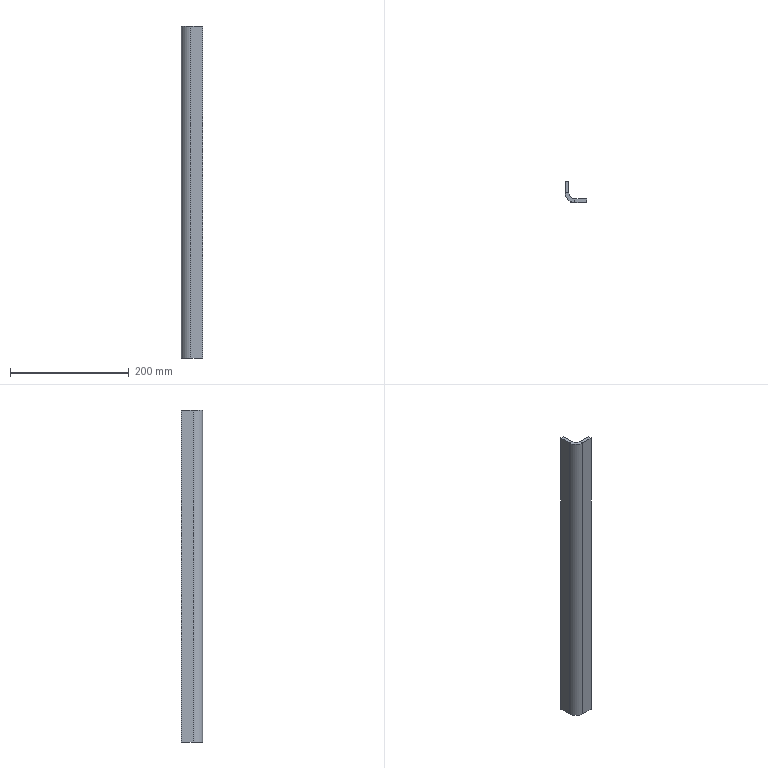Part | SolidWorks | features FlatPattern 1, SMBaseFlange 1, SheetMetal 1 | 1 solid | 14 faces | box 36 x 36 x 560 mm | volume 203012 mm3 | plane 12 | cylinder 2 | commonest cylinder face diameters 20 x1 32 x1
STEP:
#1=CARTESIAN_POINT('',(0.,16.,560.));
#2=VERTEX_POINT('',#1);
#3=CARTESIAN_POINT('',(6.,16.,560.));
#4=VERTEX_POINT('',#3);
#5=CARTESIAN_POINT('',(0.,16.,560.));
#6=DIRECTION('',(1.,0.,0.));
#7=VECTOR('',#6,1000.);
#8=LINE('',#5,#7);
#9=EDGE_CURVE('',#2,#4,#8,.T.);
#10=ORIENTED_EDGE('',*,*,#9,.F.);
#11=CARTESIAN_POINT('',(16.,0.,560.));
#12=VERTEX_POINT('',#11);
#13=CARTESIAN_POINT('',(16.,16.,560.));
#14=DIRECTION('',(0.,0.,1.));
#15=DIRECTION('',(-1.,0.,0.));
#16=AXIS2_PLACEMENT_3D('',#13,#14,#15);
#17=CIRCLE('',#16,16.);
#18=EDGE_CURVE('',#2,#12,#17,.T.);
#19=ORIENTED_EDGE('',*,*,#18,.T.);
#20=CARTESIAN_POINT('',(16.,6.,560.));
#21=VERTEX_POINT('',#20);
#22=CARTESIAN_POINT('',(16.,6.,560.));
#23=DIRECTION('',(0.,-1.,0.));
#24=VECTOR('',#23,1000.);
#25=LINE('',#22,#24);
#26=EDGE_CURVE('',#21,#12,#25,.T.);
#27=ORIENTED_EDGE('',*,*,#26,.F.);
#28=CARTESIAN_POINT('',(16.,16.,560.));
#29=DIRECTION('',(0.,0.,1.));
#30=DIRECTION('',(1.,0.,0.));
#31=AXIS2_PLACEMENT_3D('',#28,#29,#30);
#32=CIRCLE('',#31,10.);
#33=EDGE_CURVE('',#4,#21,#32,.T.);
#34=ORIENTED_EDGE('',*,*,#33,.F.);
#35=EDGE_LOOP('',(#10,#19,#27,#34));
#36=FACE_OUTER_BOUND('',#35,.T.);
#37=CARTESIAN_POINT('',(0.,16.,560.));
#38=DIRECTION('',(0.,0.,1.));
#39=DIRECTION('',(1.,0.,0.));
#40=AXIS2_PLACEMENT_3D('',#37,#38,#39);
#41=PLANE('',#40);
#42=ADVANCED_FACE('',(#36),#41,.T.);
#43=CARTESIAN_POINT('',(0.,36.,560.));
#44=VERTEX_POINT('',#43);
#45=CARTESIAN_POINT('',(0.,0.,560.));
#46=DIRECTION('',(0.,-1.,0.));
#47=VECTOR('',#46,1000.);
#48=LINE('',#45,#47);
#49=EDGE_CURVE('',#44,#2,#48,.T.);
#50=ORIENTED_EDGE('',*,*,#49,.T.);
#51=ORIENTED_EDGE('',*,*,#9,.T.);
#52=CARTESIAN_POINT('',(6.,36.,560.));
#53=VERTEX_POINT('',#52);
#54=CARTESIAN_POINT('',(6.,0.,560.));
#55=DIRECTION('',(0.,-1.,0.));
#56=VECTOR('',#55,1000.);
#57=LINE('',#54,#56);
#58=EDGE_CURVE('',#53,#4,#57,.T.);
#59=ORIENTED_EDGE('',*,*,#58,.F.);
#60=CARTESIAN_POINT('',(0.,36.,560.));
#61=DIRECTION('',(1.,0.,0.));
#62=VECTOR('',#61,1000.);
#63=LINE('',#60,#62);
#64=EDGE_CURVE('',#44,#53,#63,.T.);
#65=ORIENTED_EDGE('',*,*,#64,.F.);
#66=EDGE_LOOP('',(#50,#51,#59,#65));
#67=FACE_OUTER_BOUND('',#66,.T.);
#68=CARTESIAN_POINT('',(16.,6.,560.));
#69=DIRECTION('',(0.,0.,1.));
#70=DIRECTION('',(1.,0.,0.));
#71=AXIS2_PLACEMENT_3D('',#68,#69,#70);
#72=PLANE('',#71);
#73=ADVANCED_FACE('',(#67),#72,.T.);
#74=CARTESIAN_POINT('',(16.,0.,0.));
#75=VERTEX_POINT('',#74);
#76=CARTESIAN_POINT('',(16.,6.,0.));
#77=VERTEX_POINT('',#76);
#78=CARTESIAN_POINT('',(16.,0.,0.));
#79=DIRECTION('',(0.,1.,0.));
#80=VECTOR('',#79,1000.);
#81=LINE('',#78,#80);
#82=EDGE_CURVE('',#75,#77,#81,.T.);
#83=ORIENTED_EDGE('',*,*,#82,.F.);
#84=CARTESIAN_POINT('',(0.,16.,0.));
#85=VERTEX_POINT('',#84);
#86=CARTESIAN_POINT('',(16.,16.,0.));
#87=DIRECTION('',(0.,0.,1.));
#88=DIRECTION('',(-1.,0.,0.));
#89=AXIS2_PLACEMENT_3D('',#86,#87,#88);
#90=CIRCLE('',#89,16.);
#91=EDGE_CURVE('',#85,#75,#90,.T.);
#92=ORIENTED_EDGE('',*,*,#91,.F.);
#93=CARTESIAN_POINT('',(6.,16.,0.));
#94=VERTEX_POINT('',#93);
#95=CARTESIAN_POINT('',(6.,16.,0.));
#96=DIRECTION('',(-1.,0.,0.));
#97=VECTOR('',#96,1000.);
#98=LINE('',#95,#97);
#99=EDGE_CURVE('',#94,#85,#98,.T.);
#100=ORIENTED_EDGE('',*,*,#99,.F.);
#101=CARTESIAN_POINT('',(16.,16.,0.));
#102=DIRECTION('',(0.,0.,1.));
#103=DIRECTION('',(1.,0.,0.));
#104=AXIS2_PLACEMENT_3D('',#101,#102,#103);
#105=CIRCLE('',#104,10.);
#106=EDGE_CURVE('',#94,#77,#105,.T.);
#107=ORIENTED_EDGE('',*,*,#106,.T.);
#108=EDGE_LOOP('',(#83,#92,#100,#107));
#109=FACE_OUTER_BOUND('',#108,.T.);
#110=CARTESIAN_POINT('',(16.,0.,0.));
#111=DIRECTION('',(0.,0.,-1.));
#112=DIRECTION('',(-1.,0.,0.));
#113=AXIS2_PLACEMENT_3D('',#110,#111,#112);
#114=PLANE('',#113);
#115=ADVANCED_FACE('',(#109),#114,.T.);
#116=CARTESIAN_POINT('',(36.,0.,0.));
#117=VERTEX_POINT('',#116);
#118=CARTESIAN_POINT('',(0.,0.,0.));
#119=DIRECTION('',(1.,0.,0.));
#120=VECTOR('',#119,1000.);
#121=LINE('',#118,#120);
#122=EDGE_CURVE('',#75,#117,#121,.T.);
#123=ORIENTED_EDGE('',*,*,#122,.F.);
#124=ORIENTED_EDGE('',*,*,#82,.T.);
#125=CARTESIAN_POINT('',(36.,6.,0.));
#126=VERTEX_POINT('',#125);
#127=CARTESIAN_POINT('',(0.,6.,0.));
#128=DIRECTION('',(1.,0.,0.));
#129=VECTOR('',#128,1000.);
#130=LINE('',#127,#129);
#131=EDGE_CURVE('',#77,#126,#130,.T.);
#132=ORIENTED_EDGE('',*,*,#131,.T.);
#133=CARTESIAN_POINT('',(36.,6.,0.));
#134=DIRECTION('',(0.,-1.,0.));
#135=VECTOR('',#134,1000.);
#136=LINE('',#133,#135);
#137=EDGE_CURVE('',#126,#117,#136,.T.);
#138=ORIENTED_EDGE('',*,*,#137,.T.);
#139=EDGE_LOOP('',(#123,#124,#132,#138));
#140=FACE_OUTER_BOUND('',#139,.T.);
#141=CARTESIAN_POINT('',(6.,16.,0.));
#142=DIRECTION('',(0.,0.,-1.));
#143=DIRECTION('',(-1.,0.,0.));
#144=AXIS2_PLACEMENT_3D('',#141,#142,#143);
#145=PLANE('',#144);
#146=ADVANCED_FACE('',(#140),#145,.T.);
#147=ORIENTED_EDGE('',*,*,#122,.T.);
#148=CARTESIAN_POINT('',(36.,0.,560.));
#149=VERTEX_POINT('',#148);
#150=CARTESIAN_POINT('',(36.,0.,560.));
#151=DIRECTION('',(0.,0.,-1.));
#152=VECTOR('',#151,1000.);
#153=LINE('',#150,#152);
#154=EDGE_CURVE('',#149,#117,#153,.T.);
#155=ORIENTED_EDGE('',*,*,#154,.F.);
#156=CARTESIAN_POINT('',(0.,0.,560.));
#157=DIRECTION('',(1.,0.,0.));
#158=VECTOR('',#157,1000.);
#159=LINE('',#156,#158);
#160=EDGE_CURVE('',#12,#149,#159,.T.);
#161=ORIENTED_EDGE('',*,*,#160,.F.);
#162=CARTESIAN_POINT('',(16.,0.,560.));
#163=DIRECTION('',(0.,0.,-1.));
#164=VECTOR('',#163,1000.);
#165=LINE('',#162,#164);
#166=EDGE_CURVE('',#12,#75,#165,.T.);
#167=ORIENTED_EDGE('',*,*,#166,.T.);
#168=EDGE_LOOP('',(#147,#155,#161,#167));
#169=FACE_OUTER_BOUND('',#168,.T.);
#170=CARTESIAN_POINT('',(0.,0.,560.));
#171=DIRECTION('',(0.,1.,0.));
#172=DIRECTION('',(0.,0.,1.));
#173=AXIS2_PLACEMENT_3D('',#170,#171,#172);
#174=PLANE('',#173);
#175=ADVANCED_FACE('',(#169),#174,.F.);
#176=ORIENTED_EDGE('',*,*,#137,.F.);
#177=CARTESIAN_POINT('',(36.,6.,560.));
#178=VERTEX_POINT('',#177);
#179=CARTESIAN_POINT('',(36.,6.,560.));
#180=DIRECTION('',(0.,0.,-1.));
#181=VECTOR('',#180,1000.);
#182=LINE('',#179,#181);
#183=EDGE_CURVE('',#178,#126,#182,.T.);
#184=ORIENTED_EDGE('',*,*,#183,.F.);
#185=CARTESIAN_POINT('',(36.,6.,560.));
#186=DIRECTION('',(0.,-1.,0.));
#187=VECTOR('',#186,1000.);
#188=LINE('',#185,#187);
#189=EDGE_CURVE('',#178,#149,#188,.T.);
#190=ORIENTED_EDGE('',*,*,#189,.T.);
#191=ORIENTED_EDGE('',*,*,#154,.T.);
#192=EDGE_LOOP('',(#176,#184,#190,#191));
#193=FACE_OUTER_BOUND('',#192,.T.);
#194=CARTESIAN_POINT('',(36.,6.,560.));
#195=DIRECTION('',(1.,0.,0.));
#196=DIRECTION('',(0.,0.,-1.));
#197=AXIS2_PLACEMENT_3D('',#194,#195,#196);
#198=PLANE('',#197);
#199=ADVANCED_FACE('',(#193),#198,.T.);
#200=ORIENTED_EDGE('',*,*,#131,.F.);
#201=CARTESIAN_POINT('',(16.,6.,560.));
#202=DIRECTION('',(0.,0.,-1.));
#203=VECTOR('',#202,1000.);
#204=LINE('',#201,#203);
#205=EDGE_CURVE('',#21,#77,#204,.T.);
#206=ORIENTED_EDGE('',*,*,#205,.F.);
#207=CARTESIAN_POINT('',(0.,6.,560.));
#208=DIRECTION('',(1.,0.,0.));
#209=VECTOR('',#208,1000.);
#210=LINE('',#207,#209);
#211=EDGE_CURVE('',#21,#178,#210,.T.);
#212=ORIENTED_EDGE('',*,*,#211,.T.);
#213=ORIENTED_EDGE('',*,*,#183,.T.);
#214=EDGE_LOOP('',(#200,#206,#212,#213));
#215=FACE_OUTER_BOUND('',#214,.T.);
#216=CARTESIAN_POINT('',(0.,6.,560.));
#217=DIRECTION('',(0.,1.,0.));
#218=DIRECTION('',(0.,0.,1.));
#219=AXIS2_PLACEMENT_3D('',#216,#217,#218);
#220=PLANE('',#219);
#221=ADVANCED_FACE('',(#215),#220,.T.);
#222=ORIENTED_EDGE('',*,*,#106,.F.);
#223=CARTESIAN_POINT('',(6.,16.,560.));
#224=DIRECTION('',(0.,0.,-1.));
#225=VECTOR('',#224,1000.);
#226=LINE('',#223,#225);
#227=EDGE_CURVE('',#4,#94,#226,.T.);
#228=ORIENTED_EDGE('',*,*,#227,.F.);
#229=ORIENTED_EDGE('',*,*,#33,.T.);
#230=ORIENTED_EDGE('',*,*,#205,.T.);
#231=EDGE_LOOP('',(#222,#228,#229,#230));
#232=FACE_OUTER_BOUND('',#231,.T.);
#233=CARTESIAN_POINT('',(16.,16.,560.));
#234=DIRECTION('',(0.,0.,-1.));
#235=DIRECTION('',(-1.,0.,0.));
#236=AXIS2_PLACEMENT_3D('',#233,#234,#235);
#237=CYLINDRICAL_SURFACE('',#236,10.);
#238=ADVANCED_FACE('',(#232),#237,.F.);
#239=CARTESIAN_POINT('',(6.,36.,0.));
#240=VERTEX_POINT('',#239);
#241=CARTESIAN_POINT('',(6.,0.,0.));
#242=DIRECTION('',(0.,-1.,0.));
#243=VECTOR('',#242,1000.);
#244=LINE('',#241,#243);
#245=EDGE_CURVE('',#240,#94,#244,.T.);
#246=ORIENTED_EDGE('',*,*,#245,.F.);
#247=CARTESIAN_POINT('',(6.,36.,560.));
#248=DIRECTION('',(0.,0.,-1.));
#249=VECTOR('',#248,1000.);
#250=LINE('',#247,#249);
#251=EDGE_CURVE('',#53,#240,#250,.T.);
#252=ORIENTED_EDGE('',*,*,#251,.F.);
#253=ORIENTED_EDGE('',*,*,#58,.T.);
#254=ORIENTED_EDGE('',*,*,#227,.T.);
#255=EDGE_LOOP('',(#246,#252,#253,#254));
#256=FACE_OUTER_BOUND('',#255,.T.);
#257=CARTESIAN_POINT('',(6.,0.,560.));
#258=DIRECTION('',(1.,0.,0.));
#259=DIRECTION('',(0.,0.,-1.));
#260=AXIS2_PLACEMENT_3D('',#257,#258,#259);
#261=PLANE('',#260);
#262=ADVANCED_FACE('',(#256),#261,.T.);
#263=CARTESIAN_POINT('',(0.,36.,0.));
#264=VERTEX_POINT('',#263);
#265=CARTESIAN_POINT('',(0.,36.,0.));
#266=DIRECTION('',(1.,0.,0.));
#267=VECTOR('',#266,1000.);
#268=LINE('',#265,#267);
#269=EDGE_CURVE('',#264,#240,#268,.T.);
#270=ORIENTED_EDGE('',*,*,#269,.F.);
#271=CARTESIAN_POINT('',(0.,36.,560.));
#272=DIRECTION('',(0.,0.,-1.));
#273=VECTOR('',#272,1000.);
#274=LINE('',#271,#273);
#275=EDGE_CURVE('',#44,#264,#274,.T.);
#276=ORIENTED_EDGE('',*,*,#275,.F.);
#277=ORIENTED_EDGE('',*,*,#64,.T.);
#278=ORIENTED_EDGE('',*,*,#251,.T.);
#279=EDGE_LOOP('',(#270,#276,#277,#278));
#280=FACE_OUTER_BOUND('',#279,.T.);
#281=CARTESIAN_POINT('',(0.,36.,560.));
#282=DIRECTION('',(0.,1.,0.));
#283=DIRECTION('',(0.,0.,1.));
#284=AXIS2_PLACEMENT_3D('',#281,#282,#283);
#285=PLANE('',#284);
#286=ADVANCED_FACE('',(#280),#285,.T.);
#287=CARTESIAN_POINT('',(0.,0.,0.));
#288=DIRECTION('',(0.,-1.,0.));
#289=VECTOR('',#288,1000.);
#290=LINE('',#287,#289);
#291=EDGE_CURVE('',#264,#85,#290,.T.);
#292=ORIENTED_EDGE('',*,*,#291,.T.);
#293=CARTESIAN_POINT('',(0.,16.,560.));
#294=DIRECTION('',(0.,0.,-1.));
#295=VECTOR('',#294,1000.);
#296=LINE('',#293,#295);
#297=EDGE_CURVE('',#2,#85,#296,.T.);
#298=ORIENTED_EDGE('',*,*,#297,.F.);
#299=ORIENTED_EDGE('',*,*,#49,.F.);
#300=ORIENTED_EDGE('',*,*,#275,.T.);
#301=EDGE_LOOP('',(#292,#298,#299,#300));
#302=FACE_OUTER_BOUND('',#301,.T.);
#303=CARTESIAN_POINT('',(0.,0.,560.));
#304=DIRECTION('',(1.,0.,0.));
#305=DIRECTION('',(0.,0.,-1.));
#306=AXIS2_PLACEMENT_3D('',#303,#304,#305);
#307=PLANE('',#306);
#308=ADVANCED_FACE('',(#302),#307,.F.);
#309=ORIENTED_EDGE('',*,*,#91,.T.);
#310=ORIENTED_EDGE('',*,*,#166,.F.);
#311=ORIENTED_EDGE('',*,*,#18,.F.);
#312=ORIENTED_EDGE('',*,*,#297,.T.);
#313=EDGE_LOOP('',(#309,#310,#311,#312));
#314=FACE_OUTER_BOUND('',#313,.T.);
#315=CARTESIAN_POINT('',(16.,16.,560.));
#316=DIRECTION('',(0.,0.,-1.));
#317=DIRECTION('',(-1.,0.,0.));
#318=AXIS2_PLACEMENT_3D('',#315,#316,#317);
#319=CYLINDRICAL_SURFACE('',#318,16.);
#320=ADVANCED_FACE('',(#314),#319,.T.);
#321=ORIENTED_EDGE('',*,*,#160,.T.);
#322=ORIENTED_EDGE('',*,*,#189,.F.);
#323=ORIENTED_EDGE('',*,*,#211,.F.);
#324=ORIENTED_EDGE('',*,*,#26,.T.);
#325=EDGE_LOOP('',(#321,#322,#323,#324));
#326=FACE_OUTER_BOUND('',#325,.T.);
#327=CARTESIAN_POINT('',(16.,16.,560.));
#328=DIRECTION('',(0.,0.,1.));
#329=DIRECTION('',(1.,0.,0.));
#330=AXIS2_PLACEMENT_3D('',#327,#328,#329);
#331=PLANE('',#330);
#332=ADVANCED_FACE('',(#326),#331,.T.);
#333=ORIENTED_EDGE('',*,*,#245,.T.);
#334=ORIENTED_EDGE('',*,*,#99,.T.);
#335=ORIENTED_EDGE('',*,*,#291,.F.);
#336=ORIENTED_EDGE('',*,*,#269,.T.);
#337=EDGE_LOOP('',(#333,#334,#335,#336));
#338=FACE_OUTER_BOUND('',#337,.T.);
#339=CARTESIAN_POINT('',(16.,16.,0.));
#340=DIRECTION('',(0.,0.,1.));
#341=DIRECTION('',(1.,0.,0.));
#342=AXIS2_PLACEMENT_3D('',#339,#340,#341);
#343=PLANE('',#342);
#344=ADVANCED_FACE('',(#338),#343,.F.);
#345=CLOSED_SHELL('',(#42,#73,#115,#146,#175,#199,#221,#238,#262,#286,#308,#320,#332,#344));
#346=MANIFOLD_SOLID_BREP('',#345);
#347=CARTESIAN_POINT('',(0.,0.,0.));
#348=DIRECTION('',(0.,0.,1.));
#349=DIRECTION('',(1.,0.,0.));
#350=AXIS2_PLACEMENT_3D('',#347,#348,#349);
#351=(LENGTH_UNIT()NAMED_UNIT(*)SI_UNIT(.MILLI.,.METRE.));
#352=UNCERTAINTY_MEASURE_WITH_UNIT(LENGTH_MEASURE(0.00001),#351,'','');
#353=(NAMED_UNIT(*)PLANE_ANGLE_UNIT()SI_UNIT($,.RADIAN.));
#354=(NAMED_UNIT(*)SI_UNIT($,.STERADIAN.)SOLID_ANGLE_UNIT());
#355=(GEOMETRIC_REPRESENTATION_CONTEXT(3)GLOBAL_UNCERTAINTY_ASSIGNED_CONTEXT((#352))GLOBAL_UNIT_ASSIGNED_CONTEXT((#351,#353,#354))REPRESENTATION_CONTEXT('',''));
#356=ADVANCED_BREP_SHAPE_REPRESENTATION('',(#346,#350),#355);